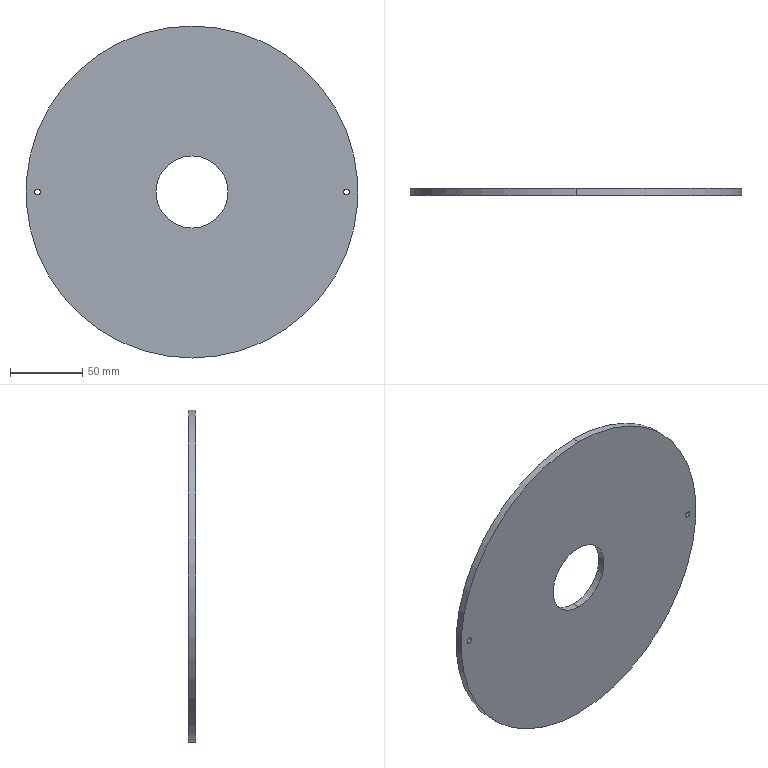Part | STEP file | Top cover | 1 solid | 10 faces | box 230 x 5 x 230 mm | volume 197795 mm3 | cylinder 8 | plane 2 | commonest cylinder face diameters 4 x4 50 x2 230 x2
STEP:
#1=CARTESIAN_POINT('',(0.,0.,-25.));
#2=VERTEX_POINT('',#1);
#3=CARTESIAN_POINT('',(0.,0.,25.));
#4=VERTEX_POINT('',#3);
#5=CARTESIAN_POINT('',(0.,0.,0.));
#6=DIRECTION('',(0.,1.,0.));
#7=DIRECTION('',(0.,0.,1.));
#8=AXIS2_PLACEMENT_3D('',#5,#6,#7);
#9=CIRCLE('',#8,25.);
#10=EDGE_CURVE('',#2,#4,#9,.T.);
#11=ORIENTED_EDGE('',*,*,#10,.F.);
#12=CARTESIAN_POINT('',(0.,5.,-25.));
#13=VERTEX_POINT('',#12);
#14=CARTESIAN_POINT('',(0.,-5.,-25.));
#15=DIRECTION('',(0.,1.,0.));
#16=VECTOR('',#15,1000.);
#17=LINE('',#14,#16);
#18=EDGE_CURVE('',#2,#13,#17,.T.);
#19=ORIENTED_EDGE('',*,*,#18,.T.);
#20=CARTESIAN_POINT('',(0.,5.,25.));
#21=VERTEX_POINT('',#20);
#22=CARTESIAN_POINT('',(0.,5.,0.));
#23=DIRECTION('',(0.,1.,0.));
#24=DIRECTION('',(0.,0.,1.));
#25=AXIS2_PLACEMENT_3D('',#22,#23,#24);
#26=CIRCLE('',#25,25.);
#27=EDGE_CURVE('',#13,#21,#26,.T.);
#28=ORIENTED_EDGE('',*,*,#27,.T.);
#29=CARTESIAN_POINT('',(0.,-5.,25.));
#30=DIRECTION('',(0.,1.,0.));
#31=VECTOR('',#30,1000.);
#32=LINE('',#29,#31);
#33=EDGE_CURVE('',#4,#21,#32,.T.);
#34=ORIENTED_EDGE('',*,*,#33,.F.);
#35=EDGE_LOOP('',(#11,#19,#28,#34));
#36=FACE_OUTER_BOUND('',#35,.T.);
#37=CARTESIAN_POINT('',(0.,-5.,0.));
#38=DIRECTION('',(0.,1.,0.));
#39=DIRECTION('',(0.,0.,1.));
#40=AXIS2_PLACEMENT_3D('',#37,#38,#39);
#41=CYLINDRICAL_SURFACE('',#40,25.);
#42=ADVANCED_FACE('',(#36),#41,.F.);
#43=CARTESIAN_POINT('',(-107.,5.,-2.));
#44=VERTEX_POINT('',#43);
#45=CARTESIAN_POINT('',(-107.,5.,2.));
#46=VERTEX_POINT('',#45);
#47=CARTESIAN_POINT('',(-107.,5.,0.));
#48=DIRECTION('',(0.,1.,0.));
#49=DIRECTION('',(0.,0.,1.));
#50=AXIS2_PLACEMENT_3D('',#47,#48,#49);
#51=CIRCLE('',#50,2.);
#52=EDGE_CURVE('',#44,#46,#51,.T.);
#53=ORIENTED_EDGE('',*,*,#52,.T.);
#54=CARTESIAN_POINT('',(-107.,0.,2.));
#55=VERTEX_POINT('',#54);
#56=CARTESIAN_POINT('',(-107.,10.,2.));
#57=DIRECTION('',(0.,-1.,0.));
#58=VECTOR('',#57,1000.);
#59=LINE('',#56,#58);
#60=EDGE_CURVE('',#46,#55,#59,.T.);
#61=ORIENTED_EDGE('',*,*,#60,.T.);
#62=CARTESIAN_POINT('',(-107.,0.,-2.));
#63=VERTEX_POINT('',#62);
#64=CARTESIAN_POINT('',(-107.,0.,0.));
#65=DIRECTION('',(0.,-1.,0.));
#66=DIRECTION('',(0.,0.,-1.));
#67=AXIS2_PLACEMENT_3D('',#64,#65,#66);
#68=CIRCLE('',#67,2.);
#69=EDGE_CURVE('',#55,#63,#68,.T.);
#70=ORIENTED_EDGE('',*,*,#69,.T.);
#71=CARTESIAN_POINT('',(-107.,10.,-2.));
#72=DIRECTION('',(0.,-1.,0.));
#73=VECTOR('',#72,1000.);
#74=LINE('',#71,#73);
#75=EDGE_CURVE('',#44,#63,#74,.T.);
#76=ORIENTED_EDGE('',*,*,#75,.F.);
#77=EDGE_LOOP('',(#53,#61,#70,#76));
#78=FACE_OUTER_BOUND('',#77,.T.);
#79=CARTESIAN_POINT('',(-107.,10.,0.));
#80=DIRECTION('',(0.,-1.,0.));
#81=DIRECTION('',(0.,0.,-1.));
#82=AXIS2_PLACEMENT_3D('',#79,#80,#81);
#83=CYLINDRICAL_SURFACE('',#82,2.);
#84=ADVANCED_FACE('',(#78),#83,.F.);
#85=CARTESIAN_POINT('',(107.,5.,-2.));
#86=VERTEX_POINT('',#85);
#87=CARTESIAN_POINT('',(107.,5.,2.));
#88=VERTEX_POINT('',#87);
#89=CARTESIAN_POINT('',(107.,5.,0.));
#90=DIRECTION('',(0.,1.,0.));
#91=DIRECTION('',(0.,0.,1.));
#92=AXIS2_PLACEMENT_3D('',#89,#90,#91);
#93=CIRCLE('',#92,2.);
#94=EDGE_CURVE('',#86,#88,#93,.T.);
#95=ORIENTED_EDGE('',*,*,#94,.T.);
#96=CARTESIAN_POINT('',(107.,0.,2.));
#97=VERTEX_POINT('',#96);
#98=CARTESIAN_POINT('',(107.,10.,2.));
#99=DIRECTION('',(0.,-1.,0.));
#100=VECTOR('',#99,1000.);
#101=LINE('',#98,#100);
#102=EDGE_CURVE('',#88,#97,#101,.T.);
#103=ORIENTED_EDGE('',*,*,#102,.T.);
#104=CARTESIAN_POINT('',(107.,0.,-2.));
#105=VERTEX_POINT('',#104);
#106=CARTESIAN_POINT('',(107.,0.,0.));
#107=DIRECTION('',(0.,-1.,0.));
#108=DIRECTION('',(0.,0.,-1.));
#109=AXIS2_PLACEMENT_3D('',#106,#107,#108);
#110=CIRCLE('',#109,2.);
#111=EDGE_CURVE('',#97,#105,#110,.T.);
#112=ORIENTED_EDGE('',*,*,#111,.T.);
#113=CARTESIAN_POINT('',(107.,10.,-2.));
#114=DIRECTION('',(0.,-1.,0.));
#115=VECTOR('',#114,1000.);
#116=LINE('',#113,#115);
#117=EDGE_CURVE('',#86,#105,#116,.T.);
#118=ORIENTED_EDGE('',*,*,#117,.F.);
#119=EDGE_LOOP('',(#95,#103,#112,#118));
#120=FACE_OUTER_BOUND('',#119,.T.);
#121=CARTESIAN_POINT('',(107.,10.,0.));
#122=DIRECTION('',(0.,-1.,0.));
#123=DIRECTION('',(0.,0.,-1.));
#124=AXIS2_PLACEMENT_3D('',#121,#122,#123);
#125=CYLINDRICAL_SURFACE('',#124,2.);
#126=ADVANCED_FACE('',(#120),#125,.F.);
#127=CARTESIAN_POINT('',(0.,5.,115.));
#128=VERTEX_POINT('',#127);
#129=CARTESIAN_POINT('',(0.,5.,-115.));
#130=VERTEX_POINT('',#129);
#131=CARTESIAN_POINT('',(0.,5.,0.));
#132=DIRECTION('',(0.,1.,0.));
#133=DIRECTION('',(0.,0.,1.));
#134=AXIS2_PLACEMENT_3D('',#131,#132,#133);
#135=CIRCLE('',#134,115.);
#136=EDGE_CURVE('',#128,#130,#135,.T.);
#137=ORIENTED_EDGE('',*,*,#136,.F.);
#138=CARTESIAN_POINT('',(0.,0.,115.));
#139=VERTEX_POINT('',#138);
#140=CARTESIAN_POINT('',(0.,5.,115.));
#141=DIRECTION('',(0.,-1.,0.));
#142=VECTOR('',#141,1000.);
#143=LINE('',#140,#142);
#144=EDGE_CURVE('',#128,#139,#143,.T.);
#145=ORIENTED_EDGE('',*,*,#144,.T.);
#146=CARTESIAN_POINT('',(0.,0.,-115.));
#147=VERTEX_POINT('',#146);
#148=CARTESIAN_POINT('',(0.,0.,0.));
#149=DIRECTION('',(0.,1.,0.));
#150=DIRECTION('',(0.,0.,1.));
#151=AXIS2_PLACEMENT_3D('',#148,#149,#150);
#152=CIRCLE('',#151,115.);
#153=EDGE_CURVE('',#139,#147,#152,.T.);
#154=ORIENTED_EDGE('',*,*,#153,.T.);
#155=CARTESIAN_POINT('',(0.,5.,-115.));
#156=DIRECTION('',(0.,-1.,0.));
#157=VECTOR('',#156,1000.);
#158=LINE('',#155,#157);
#159=EDGE_CURVE('',#130,#147,#158,.T.);
#160=ORIENTED_EDGE('',*,*,#159,.F.);
#161=EDGE_LOOP('',(#137,#145,#154,#160));
#162=FACE_OUTER_BOUND('',#161,.T.);
#163=CARTESIAN_POINT('',(0.,5.,0.));
#164=DIRECTION('',(0.,-1.,0.));
#165=DIRECTION('',(0.,0.,-1.));
#166=AXIS2_PLACEMENT_3D('',#163,#164,#165);
#167=CYLINDRICAL_SURFACE('',#166,115.);
#168=ADVANCED_FACE('',(#162),#167,.T.);
#169=ORIENTED_EDGE('',*,*,#144,.F.);
#170=CARTESIAN_POINT('',(0.,5.,0.));
#171=DIRECTION('',(0.,1.,0.));
#172=DIRECTION('',(0.,0.,1.));
#173=AXIS2_PLACEMENT_3D('',#170,#171,#172);
#174=CIRCLE('',#173,115.);
#175=EDGE_CURVE('',#130,#128,#174,.T.);
#176=ORIENTED_EDGE('',*,*,#175,.F.);
#177=ORIENTED_EDGE('',*,*,#159,.T.);
#178=CARTESIAN_POINT('',(0.,0.,0.));
#179=DIRECTION('',(0.,1.,0.));
#180=DIRECTION('',(0.,0.,1.));
#181=AXIS2_PLACEMENT_3D('',#178,#179,#180);
#182=CIRCLE('',#181,115.);
#183=EDGE_CURVE('',#147,#139,#182,.T.);
#184=ORIENTED_EDGE('',*,*,#183,.T.);
#185=EDGE_LOOP('',(#169,#176,#177,#184));
#186=FACE_OUTER_BOUND('',#185,.T.);
#187=CARTESIAN_POINT('',(0.,5.,0.));
#188=DIRECTION('',(0.,-1.,0.));
#189=DIRECTION('',(0.,0.,-1.));
#190=AXIS2_PLACEMENT_3D('',#187,#188,#189);
#191=CYLINDRICAL_SURFACE('',#190,115.);
#192=ADVANCED_FACE('',(#186),#191,.T.);
#193=CARTESIAN_POINT('',(0.,5.,0.));
#194=DIRECTION('',(0.,1.,0.));
#195=DIRECTION('',(0.,0.,1.));
#196=AXIS2_PLACEMENT_3D('',#193,#194,#195);
#197=CIRCLE('',#196,25.);
#198=EDGE_CURVE('',#21,#13,#197,.T.);
#199=ORIENTED_EDGE('',*,*,#198,.F.);
#200=ORIENTED_EDGE('',*,*,#27,.F.);
#201=EDGE_LOOP('',(#199,#200));
#202=FACE_BOUND('',#201,.T.);
#203=ORIENTED_EDGE('',*,*,#52,.F.);
#204=CARTESIAN_POINT('',(-107.,5.,0.));
#205=DIRECTION('',(0.,1.,0.));
#206=DIRECTION('',(0.,0.,1.));
#207=AXIS2_PLACEMENT_3D('',#204,#205,#206);
#208=CIRCLE('',#207,2.);
#209=EDGE_CURVE('',#46,#44,#208,.T.);
#210=ORIENTED_EDGE('',*,*,#209,.F.);
#211=EDGE_LOOP('',(#203,#210));
#212=FACE_BOUND('',#211,.T.);
#213=ORIENTED_EDGE('',*,*,#94,.F.);
#214=CARTESIAN_POINT('',(107.,5.,0.));
#215=DIRECTION('',(0.,1.,0.));
#216=DIRECTION('',(0.,0.,1.));
#217=AXIS2_PLACEMENT_3D('',#214,#215,#216);
#218=CIRCLE('',#217,2.);
#219=EDGE_CURVE('',#88,#86,#218,.T.);
#220=ORIENTED_EDGE('',*,*,#219,.F.);
#221=EDGE_LOOP('',(#213,#220));
#222=FACE_BOUND('',#221,.T.);
#223=ORIENTED_EDGE('',*,*,#175,.T.);
#224=ORIENTED_EDGE('',*,*,#136,.T.);
#225=EDGE_LOOP('',(#223,#224));
#226=FACE_OUTER_BOUND('',#225,.T.);
#227=CARTESIAN_POINT('',(0.,5.,0.));
#228=DIRECTION('',(0.,1.,0.));
#229=DIRECTION('',(0.,0.,1.));
#230=AXIS2_PLACEMENT_3D('',#227,#228,#229);
#231=PLANE('',#230);
#232=ADVANCED_FACE('',(#202,#212,#222,#226),#231,.T.);
#233=CARTESIAN_POINT('',(0.,0.,0.));
#234=DIRECTION('',(0.,1.,0.));
#235=DIRECTION('',(0.,0.,1.));
#236=AXIS2_PLACEMENT_3D('',#233,#234,#235);
#237=CIRCLE('',#236,25.);
#238=EDGE_CURVE('',#4,#2,#237,.T.);
#239=ORIENTED_EDGE('',*,*,#238,.T.);
#240=ORIENTED_EDGE('',*,*,#10,.T.);
#241=EDGE_LOOP('',(#239,#240));
#242=FACE_BOUND('',#241,.T.);
#243=CARTESIAN_POINT('',(-107.,0.,0.));
#244=DIRECTION('',(0.,-1.,0.));
#245=DIRECTION('',(0.,0.,-1.));
#246=AXIS2_PLACEMENT_3D('',#243,#244,#245);
#247=CIRCLE('',#246,2.);
#248=EDGE_CURVE('',#63,#55,#247,.T.);
#249=ORIENTED_EDGE('',*,*,#248,.F.);
#250=ORIENTED_EDGE('',*,*,#69,.F.);
#251=EDGE_LOOP('',(#249,#250));
#252=FACE_BOUND('',#251,.T.);
#253=CARTESIAN_POINT('',(107.,0.,0.));
#254=DIRECTION('',(0.,-1.,0.));
#255=DIRECTION('',(0.,0.,-1.));
#256=AXIS2_PLACEMENT_3D('',#253,#254,#255);
#257=CIRCLE('',#256,2.);
#258=EDGE_CURVE('',#105,#97,#257,.T.);
#259=ORIENTED_EDGE('',*,*,#258,.F.);
#260=ORIENTED_EDGE('',*,*,#111,.F.);
#261=EDGE_LOOP('',(#259,#260));
#262=FACE_BOUND('',#261,.T.);
#263=ORIENTED_EDGE('',*,*,#183,.F.);
#264=ORIENTED_EDGE('',*,*,#153,.F.);
#265=EDGE_LOOP('',(#263,#264));
#266=FACE_OUTER_BOUND('',#265,.T.);
#267=CARTESIAN_POINT('',(0.,0.,0.));
#268=DIRECTION('',(0.,1.,0.));
#269=DIRECTION('',(0.,0.,1.));
#270=AXIS2_PLACEMENT_3D('',#267,#268,#269);
#271=PLANE('',#270);
#272=ADVANCED_FACE('',(#242,#252,#262,#266),#271,.F.);
#273=ORIENTED_EDGE('',*,*,#102,.F.);
#274=ORIENTED_EDGE('',*,*,#219,.T.);
#275=ORIENTED_EDGE('',*,*,#117,.T.);
#276=ORIENTED_EDGE('',*,*,#258,.T.);
#277=EDGE_LOOP('',(#273,#274,#275,#276));
#278=FACE_OUTER_BOUND('',#277,.T.);
#279=CARTESIAN_POINT('',(107.,10.,0.));
#280=DIRECTION('',(0.,-1.,0.));
#281=DIRECTION('',(0.,0.,-1.));
#282=AXIS2_PLACEMENT_3D('',#279,#280,#281);
#283=CYLINDRICAL_SURFACE('',#282,2.);
#284=ADVANCED_FACE('',(#278),#283,.F.);
#285=ORIENTED_EDGE('',*,*,#60,.F.);
#286=ORIENTED_EDGE('',*,*,#209,.T.);
#287=ORIENTED_EDGE('',*,*,#75,.T.);
#288=ORIENTED_EDGE('',*,*,#248,.T.);
#289=EDGE_LOOP('',(#285,#286,#287,#288));
#290=FACE_OUTER_BOUND('',#289,.T.);
#291=CARTESIAN_POINT('',(-107.,10.,0.));
#292=DIRECTION('',(0.,-1.,0.));
#293=DIRECTION('',(0.,0.,-1.));
#294=AXIS2_PLACEMENT_3D('',#291,#292,#293);
#295=CYLINDRICAL_SURFACE('',#294,2.);
#296=ADVANCED_FACE('',(#290),#295,.F.);
#297=ORIENTED_EDGE('',*,*,#18,.F.);
#298=ORIENTED_EDGE('',*,*,#238,.F.);
#299=ORIENTED_EDGE('',*,*,#33,.T.);
#300=ORIENTED_EDGE('',*,*,#198,.T.);
#301=EDGE_LOOP('',(#297,#298,#299,#300));
#302=FACE_OUTER_BOUND('',#301,.T.);
#303=CARTESIAN_POINT('',(0.,-5.,0.));
#304=DIRECTION('',(0.,1.,0.));
#305=DIRECTION('',(0.,0.,1.));
#306=AXIS2_PLACEMENT_3D('',#303,#304,#305);
#307=CYLINDRICAL_SURFACE('',#306,25.);
#308=ADVANCED_FACE('',(#302),#307,.F.);
#309=CLOSED_SHELL('',(#42,#84,#126,#168,#192,#232,#272,#284,#296,#308));
#310=MANIFOLD_SOLID_BREP('',#309);
#311=CARTESIAN_POINT('',(0.,0.,0.));
#312=DIRECTION('',(0.,0.,1.));
#313=DIRECTION('',(1.,0.,0.));
#314=AXIS2_PLACEMENT_3D('',#311,#312,#313);
#315=(LENGTH_UNIT()NAMED_UNIT(*)SI_UNIT(.MILLI.,.METRE.));
#316=UNCERTAINTY_MEASURE_WITH_UNIT(LENGTH_MEASURE(0.00001),#315,'','');
#317=(NAMED_UNIT(*)PLANE_ANGLE_UNIT()SI_UNIT($,.RADIAN.));
#318=(NAMED_UNIT(*)SI_UNIT($,.STERADIAN.)SOLID_ANGLE_UNIT());
#319=(GEOMETRIC_REPRESENTATION_CONTEXT(3)GLOBAL_UNCERTAINTY_ASSIGNED_CONTEXT((#316))GLOBAL_UNIT_ASSIGNED_CONTEXT((#315,#317,#318))REPRESENTATION_CONTEXT('',''));
#320=ADVANCED_BREP_SHAPE_REPRESENTATION('',(#310,#314),#319);